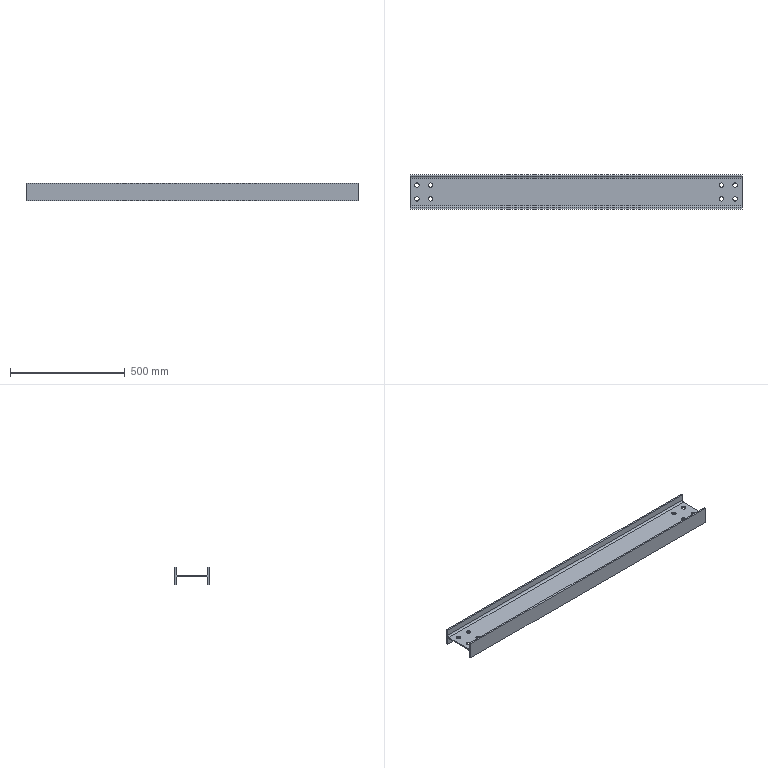Part | STEP file | Powder bin secondary beam 9 body_Default<As Machined> | 1 solid | 34 faces | box 1445 x 150 x 75 mm | volume 2567894 mm3 | cylinder 20 | plane 14 | commonest cylinder face diameters 19 x16 16 x4